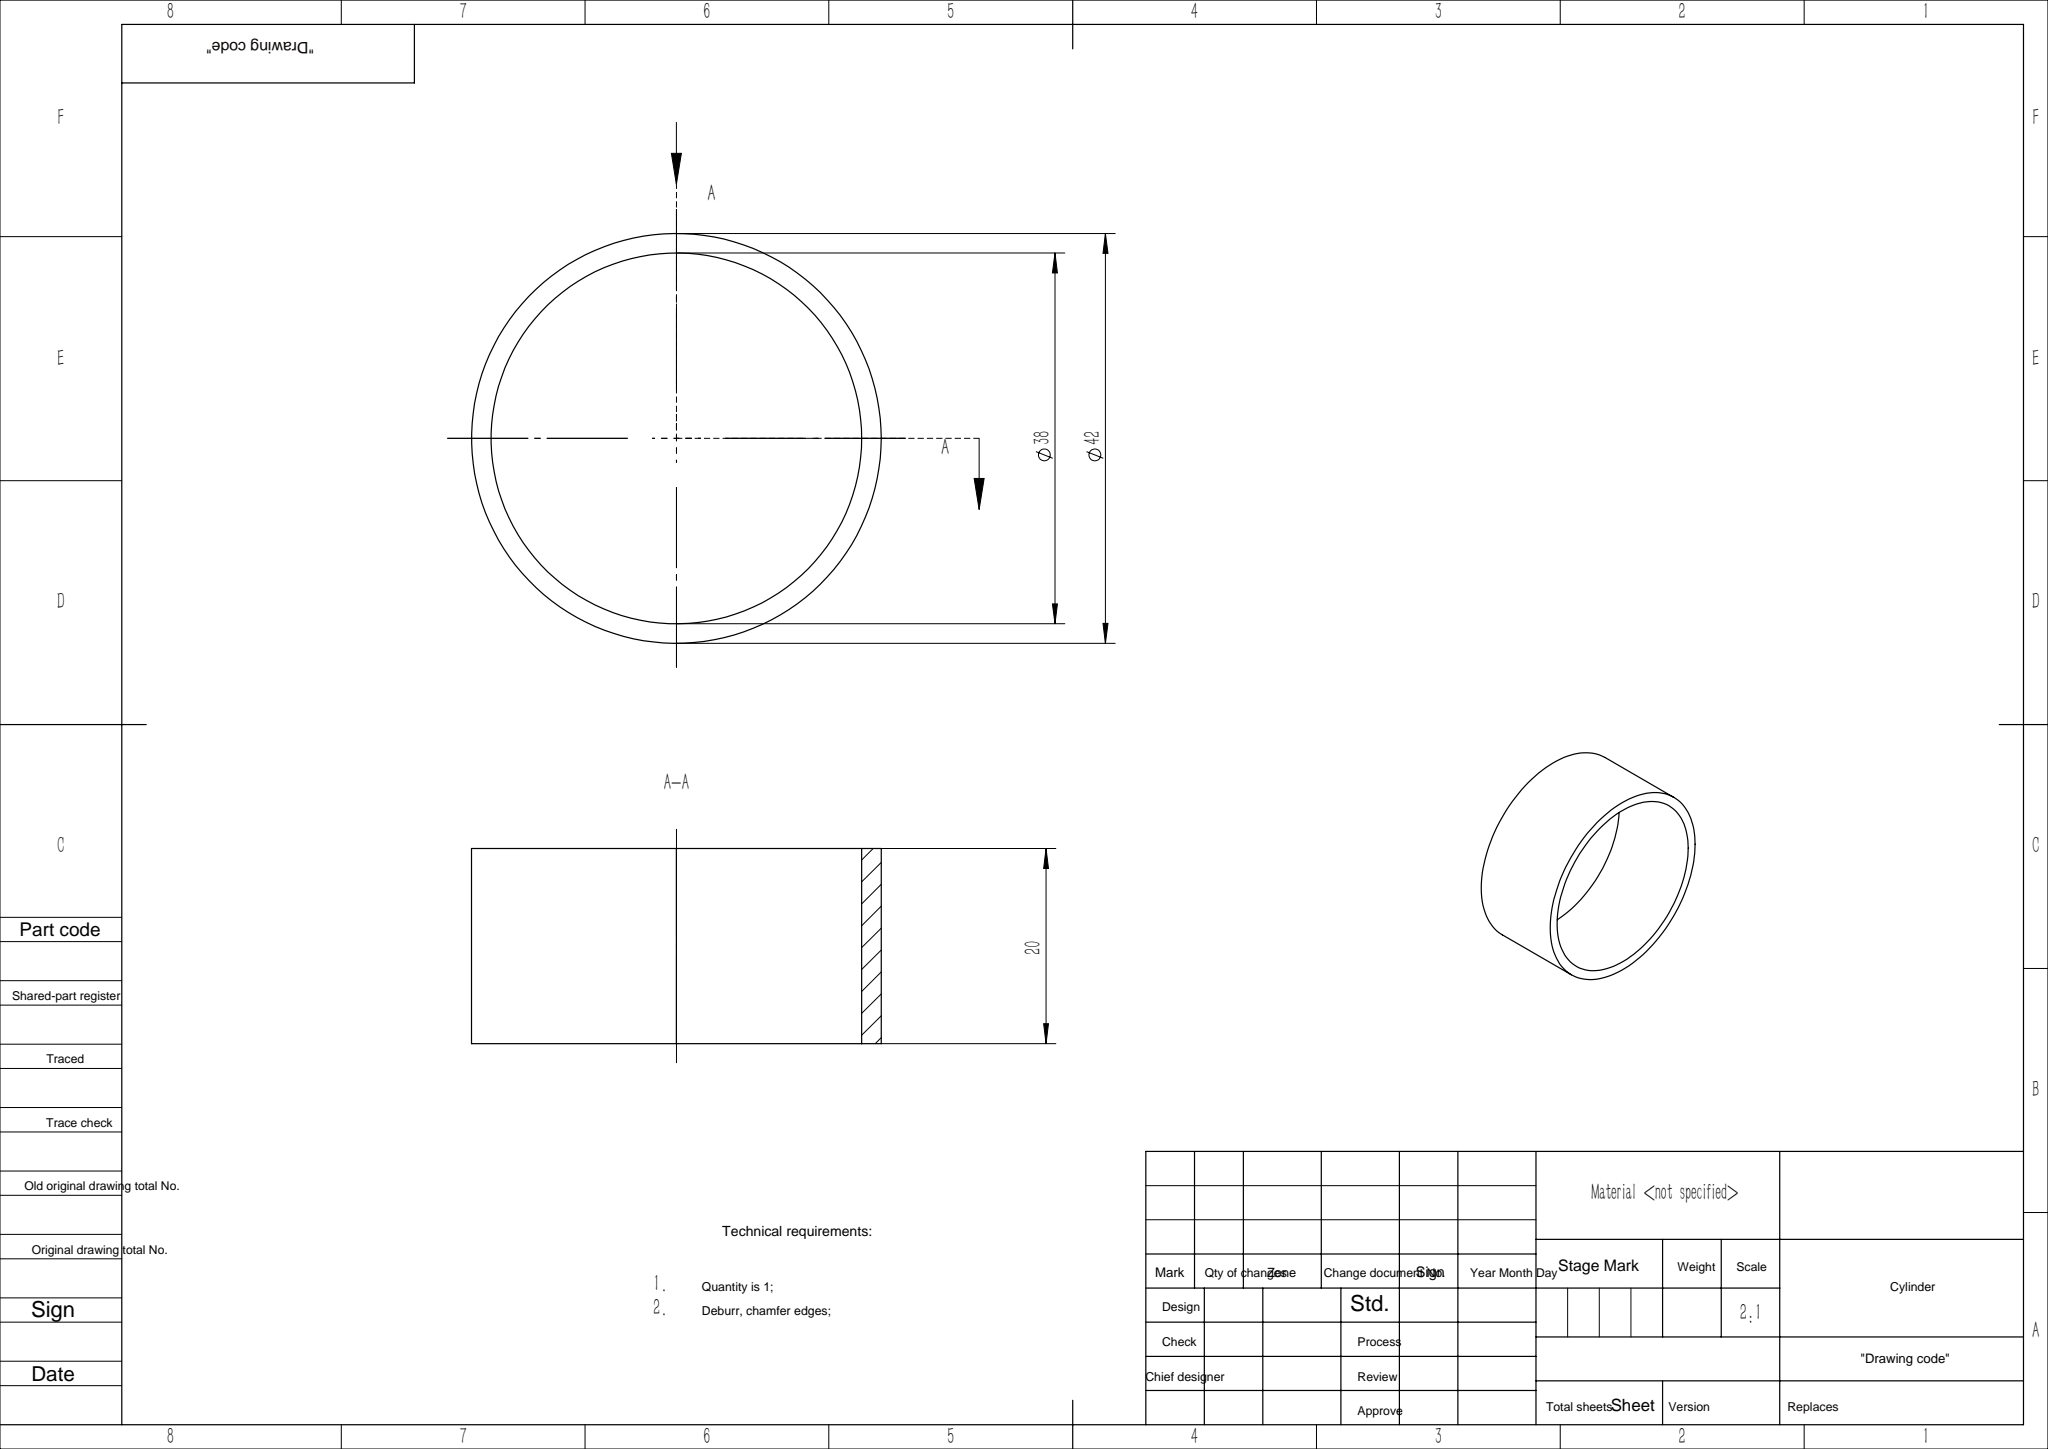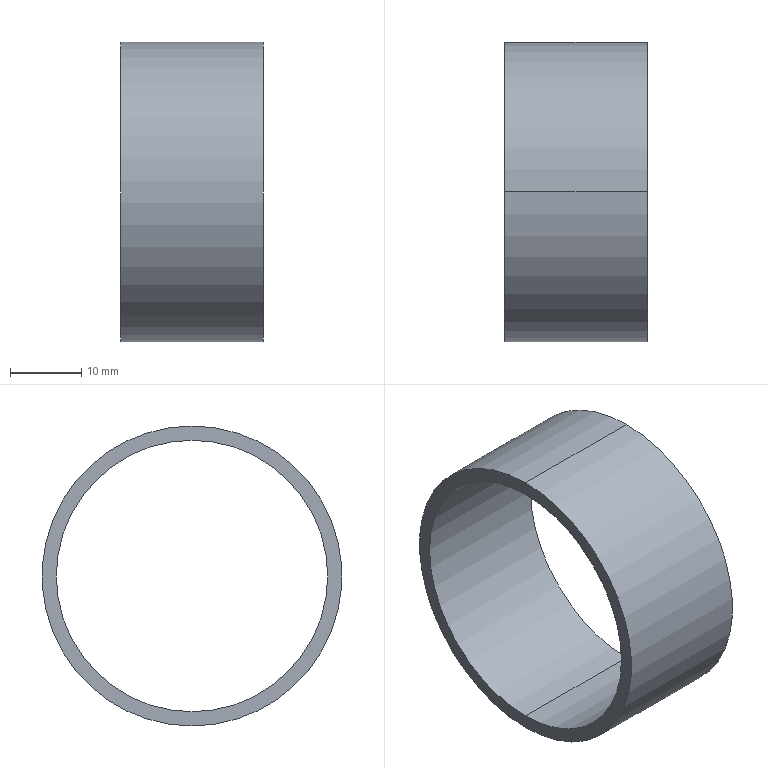Part | SolidWorks | features Extrusion 1 | 1 solid | 6 faces | box 20 x 42 x 42 mm | volume 5027 mm3 | cylinder 4 | plane 2 | commonest cylinder face diameters 38 x2 42 x2
STEP:
#1=CARTESIAN_POINT('',(649.7,-379.,-182.));
#2=VERTEX_POINT('',#1);
#3=CARTESIAN_POINT('',(649.7,-379.,-220.));
#4=VERTEX_POINT('',#3);
#5=CARTESIAN_POINT('',(649.7,-379.,-201.));
#6=DIRECTION('',(1.,0.,0.));
#7=DIRECTION('',(0.,0.,-1.));
#8=AXIS2_PLACEMENT_3D('',#5,#6,#7);
#9=CIRCLE('',#8,19.);
#10=EDGE_CURVE('',#2,#4,#9,.T.);
#11=ORIENTED_EDGE('',*,*,#10,.T.);
#12=CARTESIAN_POINT('',(629.7,-379.,-220.));
#13=VERTEX_POINT('',#12);
#14=CARTESIAN_POINT('',(649.7,-379.,-220.));
#15=DIRECTION('',(-1.,0.,0.));
#16=VECTOR('',#15,1000.);
#17=LINE('',#14,#16);
#18=EDGE_CURVE('',#4,#13,#17,.T.);
#19=ORIENTED_EDGE('',*,*,#18,.T.);
#20=CARTESIAN_POINT('',(629.7,-379.,-182.));
#21=VERTEX_POINT('',#20);
#22=CARTESIAN_POINT('',(629.7,-379.,-201.));
#23=DIRECTION('',(1.,0.,0.));
#24=DIRECTION('',(0.,0.,-1.));
#25=AXIS2_PLACEMENT_3D('',#22,#23,#24);
#26=CIRCLE('',#25,19.);
#27=EDGE_CURVE('',#21,#13,#26,.T.);
#28=ORIENTED_EDGE('',*,*,#27,.F.);
#29=CARTESIAN_POINT('',(649.7,-379.,-182.));
#30=DIRECTION('',(-1.,0.,0.));
#31=VECTOR('',#30,1000.);
#32=LINE('',#29,#31);
#33=EDGE_CURVE('',#2,#21,#32,.T.);
#34=ORIENTED_EDGE('',*,*,#33,.F.);
#35=EDGE_LOOP('',(#11,#19,#28,#34));
#36=FACE_OUTER_BOUND('',#35,.T.);
#37=CARTESIAN_POINT('',(649.7,-379.,-201.));
#38=DIRECTION('',(-1.,0.,0.));
#39=DIRECTION('',(0.,0.,1.));
#40=AXIS2_PLACEMENT_3D('',#37,#38,#39);
#41=CYLINDRICAL_SURFACE('',#40,19.);
#42=ADVANCED_FACE('',(#36),#41,.F.);
#43=CARTESIAN_POINT('',(649.7,-379.,-222.));
#44=VERTEX_POINT('',#43);
#45=CARTESIAN_POINT('',(649.7,-379.,-180.));
#46=VERTEX_POINT('',#45);
#47=CARTESIAN_POINT('',(649.7,-379.,-201.));
#48=DIRECTION('',(1.,0.,0.));
#49=DIRECTION('',(0.,0.,-1.));
#50=AXIS2_PLACEMENT_3D('',#47,#48,#49);
#51=CIRCLE('',#50,21.);
#52=EDGE_CURVE('',#44,#46,#51,.T.);
#53=ORIENTED_EDGE('',*,*,#52,.F.);
#54=CARTESIAN_POINT('',(629.7,-379.,-222.));
#55=VERTEX_POINT('',#54);
#56=CARTESIAN_POINT('',(649.7,-379.,-222.));
#57=DIRECTION('',(-1.,0.,0.));
#58=VECTOR('',#57,1000.);
#59=LINE('',#56,#58);
#60=EDGE_CURVE('',#44,#55,#59,.T.);
#61=ORIENTED_EDGE('',*,*,#60,.T.);
#62=CARTESIAN_POINT('',(629.7,-379.,-180.));
#63=VERTEX_POINT('',#62);
#64=CARTESIAN_POINT('',(629.7,-379.,-201.));
#65=DIRECTION('',(1.,0.,0.));
#66=DIRECTION('',(0.,0.,-1.));
#67=AXIS2_PLACEMENT_3D('',#64,#65,#66);
#68=CIRCLE('',#67,21.);
#69=EDGE_CURVE('',#55,#63,#68,.T.);
#70=ORIENTED_EDGE('',*,*,#69,.T.);
#71=CARTESIAN_POINT('',(649.7,-379.,-180.));
#72=DIRECTION('',(-1.,0.,0.));
#73=VECTOR('',#72,1000.);
#74=LINE('',#71,#73);
#75=EDGE_CURVE('',#46,#63,#74,.T.);
#76=ORIENTED_EDGE('',*,*,#75,.F.);
#77=EDGE_LOOP('',(#53,#61,#70,#76));
#78=FACE_OUTER_BOUND('',#77,.T.);
#79=CARTESIAN_POINT('',(649.7,-379.,-201.));
#80=DIRECTION('',(-1.,0.,0.));
#81=DIRECTION('',(0.,0.,1.));
#82=AXIS2_PLACEMENT_3D('',#79,#80,#81);
#83=CYLINDRICAL_SURFACE('',#82,21.);
#84=ADVANCED_FACE('',(#78),#83,.T.);
#85=CARTESIAN_POINT('',(649.7,-379.,-201.));
#86=DIRECTION('',(1.,0.,0.));
#87=DIRECTION('',(0.,0.,-1.));
#88=AXIS2_PLACEMENT_3D('',#85,#86,#87);
#89=CIRCLE('',#88,21.);
#90=EDGE_CURVE('',#46,#44,#89,.T.);
#91=ORIENTED_EDGE('',*,*,#90,.T.);
#92=ORIENTED_EDGE('',*,*,#52,.T.);
#93=EDGE_LOOP('',(#91,#92));
#94=FACE_OUTER_BOUND('',#93,.T.);
#95=ORIENTED_EDGE('',*,*,#10,.F.);
#96=CARTESIAN_POINT('',(649.7,-379.,-201.));
#97=DIRECTION('',(1.,0.,0.));
#98=DIRECTION('',(0.,0.,-1.));
#99=AXIS2_PLACEMENT_3D('',#96,#97,#98);
#100=CIRCLE('',#99,19.);
#101=EDGE_CURVE('',#4,#2,#100,.T.);
#102=ORIENTED_EDGE('',*,*,#101,.F.);
#103=EDGE_LOOP('',(#95,#102));
#104=FACE_BOUND('',#103,.T.);
#105=CARTESIAN_POINT('',(649.7,-379.,-201.));
#106=DIRECTION('',(1.,0.,0.));
#107=DIRECTION('',(0.,0.,-1.));
#108=AXIS2_PLACEMENT_3D('',#105,#106,#107);
#109=PLANE('',#108);
#110=ADVANCED_FACE('',(#94,#104),#109,.T.);
#111=CARTESIAN_POINT('',(629.7,-379.,-201.));
#112=DIRECTION('',(1.,0.,0.));
#113=DIRECTION('',(0.,0.,-1.));
#114=AXIS2_PLACEMENT_3D('',#111,#112,#113);
#115=CIRCLE('',#114,21.);
#116=EDGE_CURVE('',#63,#55,#115,.T.);
#117=ORIENTED_EDGE('',*,*,#116,.F.);
#118=ORIENTED_EDGE('',*,*,#69,.F.);
#119=EDGE_LOOP('',(#117,#118));
#120=FACE_OUTER_BOUND('',#119,.T.);
#121=ORIENTED_EDGE('',*,*,#27,.T.);
#122=CARTESIAN_POINT('',(629.7,-379.,-201.));
#123=DIRECTION('',(1.,0.,0.));
#124=DIRECTION('',(0.,0.,-1.));
#125=AXIS2_PLACEMENT_3D('',#122,#123,#124);
#126=CIRCLE('',#125,19.);
#127=EDGE_CURVE('',#13,#21,#126,.T.);
#128=ORIENTED_EDGE('',*,*,#127,.T.);
#129=EDGE_LOOP('',(#121,#128));
#130=FACE_BOUND('',#129,.T.);
#131=CARTESIAN_POINT('',(629.7,-379.,-201.));
#132=DIRECTION('',(1.,0.,0.));
#133=DIRECTION('',(0.,0.,-1.));
#134=AXIS2_PLACEMENT_3D('',#131,#132,#133);
#135=PLANE('',#134);
#136=ADVANCED_FACE('',(#120,#130),#135,.F.);
#137=ORIENTED_EDGE('',*,*,#60,.F.);
#138=ORIENTED_EDGE('',*,*,#90,.F.);
#139=ORIENTED_EDGE('',*,*,#75,.T.);
#140=ORIENTED_EDGE('',*,*,#116,.T.);
#141=EDGE_LOOP('',(#137,#138,#139,#140));
#142=FACE_OUTER_BOUND('',#141,.T.);
#143=CARTESIAN_POINT('',(649.7,-379.,-201.));
#144=DIRECTION('',(-1.,0.,0.));
#145=DIRECTION('',(0.,0.,1.));
#146=AXIS2_PLACEMENT_3D('',#143,#144,#145);
#147=CYLINDRICAL_SURFACE('',#146,21.);
#148=ADVANCED_FACE('',(#142),#147,.T.);
#149=ORIENTED_EDGE('',*,*,#18,.F.);
#150=ORIENTED_EDGE('',*,*,#101,.T.);
#151=ORIENTED_EDGE('',*,*,#33,.T.);
#152=ORIENTED_EDGE('',*,*,#127,.F.);
#153=EDGE_LOOP('',(#149,#150,#151,#152));
#154=FACE_OUTER_BOUND('',#153,.T.);
#155=CARTESIAN_POINT('',(649.7,-379.,-201.));
#156=DIRECTION('',(-1.,0.,0.));
#157=DIRECTION('',(0.,0.,1.));
#158=AXIS2_PLACEMENT_3D('',#155,#156,#157);
#159=CYLINDRICAL_SURFACE('',#158,19.);
#160=ADVANCED_FACE('',(#154),#159,.F.);
#161=CLOSED_SHELL('',(#42,#84,#110,#136,#148,#160));
#162=MANIFOLD_SOLID_BREP('',#161);
#163=CARTESIAN_POINT('',(0.,0.,0.));
#164=DIRECTION('',(0.,0.,1.));
#165=DIRECTION('',(1.,0.,0.));
#166=AXIS2_PLACEMENT_3D('',#163,#164,#165);
#167=(LENGTH_UNIT()NAMED_UNIT(*)SI_UNIT(.MILLI.,.METRE.));
#168=UNCERTAINTY_MEASURE_WITH_UNIT(LENGTH_MEASURE(0.00001),#167,'','');
#169=(NAMED_UNIT(*)PLANE_ANGLE_UNIT()SI_UNIT($,.RADIAN.));
#170=(NAMED_UNIT(*)SI_UNIT($,.STERADIAN.)SOLID_ANGLE_UNIT());
#171=(GEOMETRIC_REPRESENTATION_CONTEXT(3)GLOBAL_UNCERTAINTY_ASSIGNED_CONTEXT((#168))GLOBAL_UNIT_ASSIGNED_CONTEXT((#167,#169,#170))REPRESENTATION_CONTEXT('',''));
#172=ADVANCED_BREP_SHAPE_REPRESENTATION('',(#162,#166),#171);